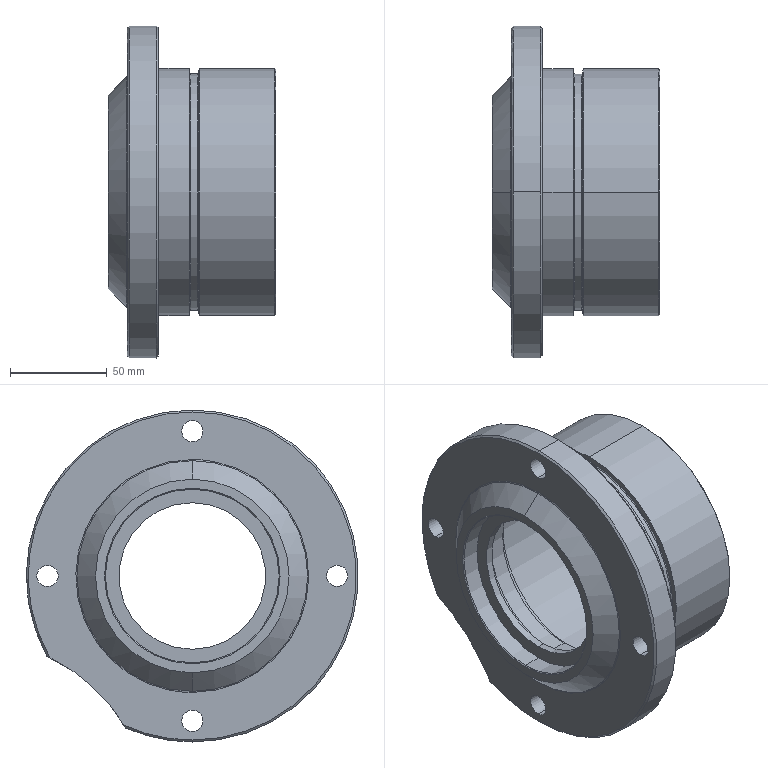Part | SolidWorks | features BaseBody 1 | 1 solid | 78 faces | box 86.84 x 172 x 172 mm | volume 513296 mm3 | cylinder 32 | spline 18 | cone 18 | plane 10 | commonest cylinder face diameters 11 x8 90 x4 110 x4 128 x4 172 x3 76 x2